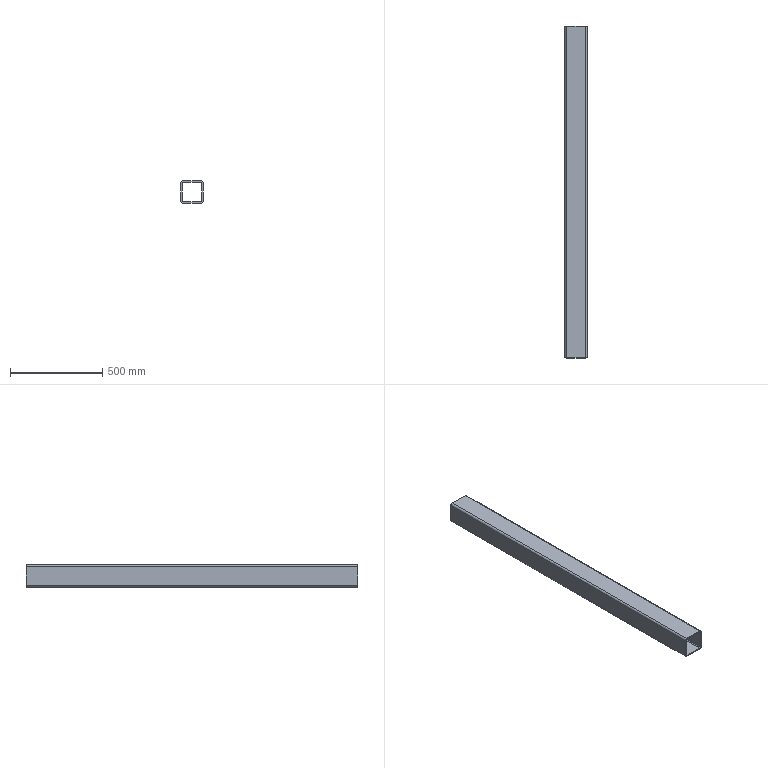Part | SolidWorks | features Extrusion 1 | 1 solid | 18 faces | box 120 x 1800 x 120 mm | volume 4795009 mm3 | plane 10 | cylinder 8 | commonest cylinder face diameters 8 x4 20 x4
STEP:
#1=CARTESIAN_POINT('',(-60.,1800.,50.));
#2=VERTEX_POINT('',#1);
#3=CARTESIAN_POINT('',(-50.,1800.,60.));
#4=VERTEX_POINT('',#3);
#5=CARTESIAN_POINT('',(-50.,1800.,50.));
#6=DIRECTION('',(0.,1.,0.));
#7=DIRECTION('',(0.,0.,-1.));
#8=AXIS2_PLACEMENT_3D('',#5,#6,#7);
#9=CIRCLE('',#8,10.);
#10=EDGE_CURVE('',#2,#4,#9,.T.);
#11=ORIENTED_EDGE('',*,*,#10,.T.);
#12=CARTESIAN_POINT('',(50.,1800.,60.));
#13=VERTEX_POINT('',#12);
#14=CARTESIAN_POINT('',(-50.,1800.,60.));
#15=DIRECTION('',(1.,0.,0.));
#16=VECTOR('',#15,1000.);
#17=LINE('',#14,#16);
#18=EDGE_CURVE('',#4,#13,#17,.T.);
#19=ORIENTED_EDGE('',*,*,#18,.T.);
#20=CARTESIAN_POINT('',(60.,1800.,50.));
#21=VERTEX_POINT('',#20);
#22=CARTESIAN_POINT('',(50.,1800.,50.));
#23=DIRECTION('',(0.,1.,0.));
#24=DIRECTION('',(0.,0.,1.));
#25=AXIS2_PLACEMENT_3D('',#22,#23,#24);
#26=CIRCLE('',#25,10.);
#27=EDGE_CURVE('',#13,#21,#26,.T.);
#28=ORIENTED_EDGE('',*,*,#27,.T.);
#29=CARTESIAN_POINT('',(60.,1800.,-50.));
#30=VERTEX_POINT('',#29);
#31=CARTESIAN_POINT('',(60.,1800.,50.));
#32=DIRECTION('',(0.,0.,-1.));
#33=VECTOR('',#32,1000.);
#34=LINE('',#31,#33);
#35=EDGE_CURVE('',#21,#30,#34,.T.);
#36=ORIENTED_EDGE('',*,*,#35,.T.);
#37=CARTESIAN_POINT('',(50.,1800.,-60.));
#38=VERTEX_POINT('',#37);
#39=CARTESIAN_POINT('',(50.,1800.,-50.));
#40=DIRECTION('',(0.,1.,0.));
#41=DIRECTION('',(0.,0.,-1.));
#42=AXIS2_PLACEMENT_3D('',#39,#40,#41);
#43=CIRCLE('',#42,10.);
#44=EDGE_CURVE('',#30,#38,#43,.T.);
#45=ORIENTED_EDGE('',*,*,#44,.T.);
#46=CARTESIAN_POINT('',(-50.,1800.,-60.));
#47=VERTEX_POINT('',#46);
#48=CARTESIAN_POINT('',(-50.,1800.,-60.));
#49=DIRECTION('',(-1.,0.,0.));
#50=VECTOR('',#49,1000.);
#51=LINE('',#48,#50);
#52=EDGE_CURVE('',#38,#47,#51,.T.);
#53=ORIENTED_EDGE('',*,*,#52,.T.);
#54=CARTESIAN_POINT('',(-60.,1800.,-50.));
#55=VERTEX_POINT('',#54);
#56=CARTESIAN_POINT('',(-50.,1800.,-50.));
#57=DIRECTION('',(0.,1.,0.));
#58=DIRECTION('',(0.,0.,-1.));
#59=AXIS2_PLACEMENT_3D('',#56,#57,#58);
#60=CIRCLE('',#59,10.);
#61=EDGE_CURVE('',#47,#55,#60,.T.);
#62=ORIENTED_EDGE('',*,*,#61,.T.);
#63=CARTESIAN_POINT('',(-60.,1800.,50.));
#64=DIRECTION('',(0.,0.,1.));
#65=VECTOR('',#64,1000.);
#66=LINE('',#63,#65);
#67=EDGE_CURVE('',#55,#2,#66,.T.);
#68=ORIENTED_EDGE('',*,*,#67,.T.);
#69=EDGE_LOOP('',(#11,#19,#28,#36,#45,#53,#62,#68));
#70=FACE_OUTER_BOUND('',#69,.T.);
#71=CARTESIAN_POINT('',(-54.,1800.,50.));
#72=VERTEX_POINT('',#71);
#73=CARTESIAN_POINT('',(-50.,1800.,54.));
#74=VERTEX_POINT('',#73);
#75=CARTESIAN_POINT('',(-50.,1800.,50.));
#76=DIRECTION('',(0.,1.,0.));
#77=DIRECTION('',(0.,0.,-1.));
#78=AXIS2_PLACEMENT_3D('',#75,#76,#77);
#79=CIRCLE('',#78,4.);
#80=EDGE_CURVE('',#72,#74,#79,.T.);
#81=ORIENTED_EDGE('',*,*,#80,.F.);
#82=CARTESIAN_POINT('',(-54.,1800.,-50.));
#83=VERTEX_POINT('',#82);
#84=CARTESIAN_POINT('',(-54.,1800.,50.));
#85=DIRECTION('',(0.,0.,1.));
#86=VECTOR('',#85,1000.);
#87=LINE('',#84,#86);
#88=EDGE_CURVE('',#83,#72,#87,.T.);
#89=ORIENTED_EDGE('',*,*,#88,.F.);
#90=CARTESIAN_POINT('',(-50.,1800.,-54.));
#91=VERTEX_POINT('',#90);
#92=CARTESIAN_POINT('',(-50.,1800.,-50.));
#93=DIRECTION('',(0.,1.,0.));
#94=DIRECTION('',(0.,0.,-1.));
#95=AXIS2_PLACEMENT_3D('',#92,#93,#94);
#96=CIRCLE('',#95,4.);
#97=EDGE_CURVE('',#91,#83,#96,.T.);
#98=ORIENTED_EDGE('',*,*,#97,.F.);
#99=CARTESIAN_POINT('',(50.,1800.,-54.));
#100=VERTEX_POINT('',#99);
#101=CARTESIAN_POINT('',(-50.,1800.,-54.));
#102=DIRECTION('',(-1.,0.,0.));
#103=VECTOR('',#102,1000.);
#104=LINE('',#101,#103);
#105=EDGE_CURVE('',#100,#91,#104,.T.);
#106=ORIENTED_EDGE('',*,*,#105,.F.);
#107=CARTESIAN_POINT('',(54.,1800.,-50.));
#108=VERTEX_POINT('',#107);
#109=CARTESIAN_POINT('',(50.,1800.,-50.));
#110=DIRECTION('',(0.,1.,0.));
#111=DIRECTION('',(0.,0.,-1.));
#112=AXIS2_PLACEMENT_3D('',#109,#110,#111);
#113=CIRCLE('',#112,4.);
#114=EDGE_CURVE('',#108,#100,#113,.T.);
#115=ORIENTED_EDGE('',*,*,#114,.F.);
#116=CARTESIAN_POINT('',(54.,1800.,50.));
#117=VERTEX_POINT('',#116);
#118=CARTESIAN_POINT('',(54.,1800.,50.));
#119=DIRECTION('',(0.,0.,-1.));
#120=VECTOR('',#119,1000.);
#121=LINE('',#118,#120);
#122=EDGE_CURVE('',#117,#108,#121,.T.);
#123=ORIENTED_EDGE('',*,*,#122,.F.);
#124=CARTESIAN_POINT('',(50.,1800.,54.));
#125=VERTEX_POINT('',#124);
#126=CARTESIAN_POINT('',(50.,1800.,50.));
#127=DIRECTION('',(0.,1.,0.));
#128=DIRECTION('',(0.,0.,1.));
#129=AXIS2_PLACEMENT_3D('',#126,#127,#128);
#130=CIRCLE('',#129,4.);
#131=EDGE_CURVE('',#125,#117,#130,.T.);
#132=ORIENTED_EDGE('',*,*,#131,.F.);
#133=CARTESIAN_POINT('',(-50.,1800.,54.));
#134=DIRECTION('',(1.,0.,0.));
#135=VECTOR('',#134,1000.);
#136=LINE('',#133,#135);
#137=EDGE_CURVE('',#74,#125,#136,.T.);
#138=ORIENTED_EDGE('',*,*,#137,.F.);
#139=EDGE_LOOP('',(#81,#89,#98,#106,#115,#123,#132,#138));
#140=FACE_BOUND('',#139,.T.);
#141=CARTESIAN_POINT('',(-50.,1800.,50.));
#142=DIRECTION('',(0.,-1.,0.));
#143=DIRECTION('',(0.,0.,-1.));
#144=AXIS2_PLACEMENT_3D('',#141,#142,#143);
#145=PLANE('',#144);
#146=ADVANCED_FACE('',(#70,#140),#145,.F.);
#147=CARTESIAN_POINT('',(-60.,0.,50.));
#148=VERTEX_POINT('',#147);
#149=CARTESIAN_POINT('',(-50.,0.,60.));
#150=VERTEX_POINT('',#149);
#151=CARTESIAN_POINT('',(-50.,0.,50.));
#152=DIRECTION('',(0.,1.,0.));
#153=DIRECTION('',(0.,0.,-1.));
#154=AXIS2_PLACEMENT_3D('',#151,#152,#153);
#155=CIRCLE('',#154,10.);
#156=EDGE_CURVE('',#148,#150,#155,.T.);
#157=ORIENTED_EDGE('',*,*,#156,.F.);
#158=CARTESIAN_POINT('',(-60.,0.,-50.));
#159=VERTEX_POINT('',#158);
#160=CARTESIAN_POINT('',(-60.,0.,50.));
#161=DIRECTION('',(0.,0.,1.));
#162=VECTOR('',#161,1000.);
#163=LINE('',#160,#162);
#164=EDGE_CURVE('',#159,#148,#163,.T.);
#165=ORIENTED_EDGE('',*,*,#164,.F.);
#166=CARTESIAN_POINT('',(-50.,0.,-60.));
#167=VERTEX_POINT('',#166);
#168=CARTESIAN_POINT('',(-50.,0.,-50.));
#169=DIRECTION('',(0.,1.,0.));
#170=DIRECTION('',(0.,0.,-1.));
#171=AXIS2_PLACEMENT_3D('',#168,#169,#170);
#172=CIRCLE('',#171,10.);
#173=EDGE_CURVE('',#167,#159,#172,.T.);
#174=ORIENTED_EDGE('',*,*,#173,.F.);
#175=CARTESIAN_POINT('',(50.,0.,-60.));
#176=VERTEX_POINT('',#175);
#177=CARTESIAN_POINT('',(-50.,0.,-60.));
#178=DIRECTION('',(-1.,0.,0.));
#179=VECTOR('',#178,1000.);
#180=LINE('',#177,#179);
#181=EDGE_CURVE('',#176,#167,#180,.T.);
#182=ORIENTED_EDGE('',*,*,#181,.F.);
#183=CARTESIAN_POINT('',(60.,0.,-50.));
#184=VERTEX_POINT('',#183);
#185=CARTESIAN_POINT('',(50.,0.,-50.));
#186=DIRECTION('',(0.,1.,0.));
#187=DIRECTION('',(0.,0.,-1.));
#188=AXIS2_PLACEMENT_3D('',#185,#186,#187);
#189=CIRCLE('',#188,10.);
#190=EDGE_CURVE('',#184,#176,#189,.T.);
#191=ORIENTED_EDGE('',*,*,#190,.F.);
#192=CARTESIAN_POINT('',(60.,0.,50.));
#193=VERTEX_POINT('',#192);
#194=CARTESIAN_POINT('',(60.,0.,50.));
#195=DIRECTION('',(0.,0.,-1.));
#196=VECTOR('',#195,1000.);
#197=LINE('',#194,#196);
#198=EDGE_CURVE('',#193,#184,#197,.T.);
#199=ORIENTED_EDGE('',*,*,#198,.F.);
#200=CARTESIAN_POINT('',(50.,0.,60.));
#201=VERTEX_POINT('',#200);
#202=CARTESIAN_POINT('',(50.,0.,50.));
#203=DIRECTION('',(0.,1.,0.));
#204=DIRECTION('',(0.,0.,1.));
#205=AXIS2_PLACEMENT_3D('',#202,#203,#204);
#206=CIRCLE('',#205,10.);
#207=EDGE_CURVE('',#201,#193,#206,.T.);
#208=ORIENTED_EDGE('',*,*,#207,.F.);
#209=CARTESIAN_POINT('',(-50.,0.,60.));
#210=DIRECTION('',(1.,0.,0.));
#211=VECTOR('',#210,1000.);
#212=LINE('',#209,#211);
#213=EDGE_CURVE('',#150,#201,#212,.T.);
#214=ORIENTED_EDGE('',*,*,#213,.F.);
#215=EDGE_LOOP('',(#157,#165,#174,#182,#191,#199,#208,#214));
#216=FACE_OUTER_BOUND('',#215,.T.);
#217=CARTESIAN_POINT('',(-54.,0.,-50.));
#218=VERTEX_POINT('',#217);
#219=CARTESIAN_POINT('',(-54.,0.,50.));
#220=VERTEX_POINT('',#219);
#221=CARTESIAN_POINT('',(-54.,0.,50.));
#222=DIRECTION('',(0.,0.,1.));
#223=VECTOR('',#222,1000.);
#224=LINE('',#221,#223);
#225=EDGE_CURVE('',#218,#220,#224,.T.);
#226=ORIENTED_EDGE('',*,*,#225,.T.);
#227=CARTESIAN_POINT('',(-50.,0.,54.));
#228=VERTEX_POINT('',#227);
#229=CARTESIAN_POINT('',(-50.,0.,50.));
#230=DIRECTION('',(0.,1.,0.));
#231=DIRECTION('',(0.,0.,-1.));
#232=AXIS2_PLACEMENT_3D('',#229,#230,#231);
#233=CIRCLE('',#232,4.);
#234=EDGE_CURVE('',#220,#228,#233,.T.);
#235=ORIENTED_EDGE('',*,*,#234,.T.);
#236=CARTESIAN_POINT('',(50.,0.,54.));
#237=VERTEX_POINT('',#236);
#238=CARTESIAN_POINT('',(-50.,0.,54.));
#239=DIRECTION('',(1.,0.,0.));
#240=VECTOR('',#239,1000.);
#241=LINE('',#238,#240);
#242=EDGE_CURVE('',#228,#237,#241,.T.);
#243=ORIENTED_EDGE('',*,*,#242,.T.);
#244=CARTESIAN_POINT('',(54.,0.,50.));
#245=VERTEX_POINT('',#244);
#246=CARTESIAN_POINT('',(50.,0.,50.));
#247=DIRECTION('',(0.,1.,0.));
#248=DIRECTION('',(0.,0.,1.));
#249=AXIS2_PLACEMENT_3D('',#246,#247,#248);
#250=CIRCLE('',#249,4.);
#251=EDGE_CURVE('',#237,#245,#250,.T.);
#252=ORIENTED_EDGE('',*,*,#251,.T.);
#253=CARTESIAN_POINT('',(54.,0.,-50.));
#254=VERTEX_POINT('',#253);
#255=CARTESIAN_POINT('',(54.,0.,50.));
#256=DIRECTION('',(0.,0.,-1.));
#257=VECTOR('',#256,1000.);
#258=LINE('',#255,#257);
#259=EDGE_CURVE('',#245,#254,#258,.T.);
#260=ORIENTED_EDGE('',*,*,#259,.T.);
#261=CARTESIAN_POINT('',(50.,0.,-54.));
#262=VERTEX_POINT('',#261);
#263=CARTESIAN_POINT('',(50.,0.,-50.));
#264=DIRECTION('',(0.,1.,0.));
#265=DIRECTION('',(0.,0.,-1.));
#266=AXIS2_PLACEMENT_3D('',#263,#264,#265);
#267=CIRCLE('',#266,4.);
#268=EDGE_CURVE('',#254,#262,#267,.T.);
#269=ORIENTED_EDGE('',*,*,#268,.T.);
#270=CARTESIAN_POINT('',(-50.,0.,-54.));
#271=VERTEX_POINT('',#270);
#272=CARTESIAN_POINT('',(-50.,0.,-54.));
#273=DIRECTION('',(-1.,0.,0.));
#274=VECTOR('',#273,1000.);
#275=LINE('',#272,#274);
#276=EDGE_CURVE('',#262,#271,#275,.T.);
#277=ORIENTED_EDGE('',*,*,#276,.T.);
#278=CARTESIAN_POINT('',(-50.,0.,-50.));
#279=DIRECTION('',(0.,1.,0.));
#280=DIRECTION('',(0.,0.,-1.));
#281=AXIS2_PLACEMENT_3D('',#278,#279,#280);
#282=CIRCLE('',#281,4.);
#283=EDGE_CURVE('',#271,#218,#282,.T.);
#284=ORIENTED_EDGE('',*,*,#283,.T.);
#285=EDGE_LOOP('',(#226,#235,#243,#252,#260,#269,#277,#284));
#286=FACE_BOUND('',#285,.T.);
#287=CARTESIAN_POINT('',(-50.,0.,50.));
#288=DIRECTION('',(0.,-1.,0.));
#289=DIRECTION('',(0.,0.,-1.));
#290=AXIS2_PLACEMENT_3D('',#287,#288,#289);
#291=PLANE('',#290);
#292=ADVANCED_FACE('',(#216,#286),#291,.T.);
#293=ORIENTED_EDGE('',*,*,#156,.T.);
#294=CARTESIAN_POINT('',(-50.,1800.,60.));
#295=DIRECTION('',(0.,-1.,0.));
#296=VECTOR('',#295,1000.);
#297=LINE('',#294,#296);
#298=EDGE_CURVE('',#4,#150,#297,.T.);
#299=ORIENTED_EDGE('',*,*,#298,.F.);
#300=ORIENTED_EDGE('',*,*,#10,.F.);
#301=CARTESIAN_POINT('',(-60.,1800.,50.));
#302=DIRECTION('',(0.,-1.,0.));
#303=VECTOR('',#302,1000.);
#304=LINE('',#301,#303);
#305=EDGE_CURVE('',#2,#148,#304,.T.);
#306=ORIENTED_EDGE('',*,*,#305,.T.);
#307=EDGE_LOOP('',(#293,#299,#300,#306));
#308=FACE_OUTER_BOUND('',#307,.T.);
#309=CARTESIAN_POINT('',(-50.,1800.,50.));
#310=DIRECTION('',(0.,-1.,0.));
#311=DIRECTION('',(0.,0.,-1.));
#312=AXIS2_PLACEMENT_3D('',#309,#310,#311);
#313=CYLINDRICAL_SURFACE('',#312,10.);
#314=ADVANCED_FACE('',(#308),#313,.T.);
#315=ORIENTED_EDGE('',*,*,#213,.T.);
#316=CARTESIAN_POINT('',(50.,1800.,60.));
#317=DIRECTION('',(0.,-1.,0.));
#318=VECTOR('',#317,1000.);
#319=LINE('',#316,#318);
#320=EDGE_CURVE('',#13,#201,#319,.T.);
#321=ORIENTED_EDGE('',*,*,#320,.F.);
#322=ORIENTED_EDGE('',*,*,#18,.F.);
#323=ORIENTED_EDGE('',*,*,#298,.T.);
#324=EDGE_LOOP('',(#315,#321,#322,#323));
#325=FACE_OUTER_BOUND('',#324,.T.);
#326=CARTESIAN_POINT('',(-50.,1800.,60.));
#327=DIRECTION('',(0.,0.,-1.));
#328=DIRECTION('',(-1.,0.,0.));
#329=AXIS2_PLACEMENT_3D('',#326,#327,#328);
#330=PLANE('',#329);
#331=ADVANCED_FACE('',(#325),#330,.F.);
#332=ORIENTED_EDGE('',*,*,#207,.T.);
#333=CARTESIAN_POINT('',(60.,1800.,50.));
#334=DIRECTION('',(0.,-1.,0.));
#335=VECTOR('',#334,1000.);
#336=LINE('',#333,#335);
#337=EDGE_CURVE('',#21,#193,#336,.T.);
#338=ORIENTED_EDGE('',*,*,#337,.F.);
#339=ORIENTED_EDGE('',*,*,#27,.F.);
#340=ORIENTED_EDGE('',*,*,#320,.T.);
#341=EDGE_LOOP('',(#332,#338,#339,#340));
#342=FACE_OUTER_BOUND('',#341,.T.);
#343=CARTESIAN_POINT('',(50.,1800.,50.));
#344=DIRECTION('',(0.,-1.,0.));
#345=DIRECTION('',(0.,0.,-1.));
#346=AXIS2_PLACEMENT_3D('',#343,#344,#345);
#347=CYLINDRICAL_SURFACE('',#346,10.);
#348=ADVANCED_FACE('',(#342),#347,.T.);
#349=ORIENTED_EDGE('',*,*,#198,.T.);
#350=CARTESIAN_POINT('',(60.,1800.,-50.));
#351=DIRECTION('',(0.,-1.,0.));
#352=VECTOR('',#351,1000.);
#353=LINE('',#350,#352);
#354=EDGE_CURVE('',#30,#184,#353,.T.);
#355=ORIENTED_EDGE('',*,*,#354,.F.);
#356=ORIENTED_EDGE('',*,*,#35,.F.);
#357=ORIENTED_EDGE('',*,*,#337,.T.);
#358=EDGE_LOOP('',(#349,#355,#356,#357));
#359=FACE_OUTER_BOUND('',#358,.T.);
#360=CARTESIAN_POINT('',(60.,1800.,50.));
#361=DIRECTION('',(-1.,0.,0.));
#362=DIRECTION('',(0.,0.,1.));
#363=AXIS2_PLACEMENT_3D('',#360,#361,#362);
#364=PLANE('',#363);
#365=ADVANCED_FACE('',(#359),#364,.F.);
#366=ORIENTED_EDGE('',*,*,#190,.T.);
#367=CARTESIAN_POINT('',(50.,1800.,-60.));
#368=DIRECTION('',(0.,-1.,0.));
#369=VECTOR('',#368,1000.);
#370=LINE('',#367,#369);
#371=EDGE_CURVE('',#38,#176,#370,.T.);
#372=ORIENTED_EDGE('',*,*,#371,.F.);
#373=ORIENTED_EDGE('',*,*,#44,.F.);
#374=ORIENTED_EDGE('',*,*,#354,.T.);
#375=EDGE_LOOP('',(#366,#372,#373,#374));
#376=FACE_OUTER_BOUND('',#375,.T.);
#377=CARTESIAN_POINT('',(50.,1800.,-50.));
#378=DIRECTION('',(0.,-1.,0.));
#379=DIRECTION('',(0.,0.,-1.));
#380=AXIS2_PLACEMENT_3D('',#377,#378,#379);
#381=CYLINDRICAL_SURFACE('',#380,10.);
#382=ADVANCED_FACE('',(#376),#381,.T.);
#383=ORIENTED_EDGE('',*,*,#181,.T.);
#384=CARTESIAN_POINT('',(-50.,1800.,-60.));
#385=DIRECTION('',(0.,-1.,0.));
#386=VECTOR('',#385,1000.);
#387=LINE('',#384,#386);
#388=EDGE_CURVE('',#47,#167,#387,.T.);
#389=ORIENTED_EDGE('',*,*,#388,.F.);
#390=ORIENTED_EDGE('',*,*,#52,.F.);
#391=ORIENTED_EDGE('',*,*,#371,.T.);
#392=EDGE_LOOP('',(#383,#389,#390,#391));
#393=FACE_OUTER_BOUND('',#392,.T.);
#394=CARTESIAN_POINT('',(-50.,1800.,-60.));
#395=DIRECTION('',(0.,0.,1.));
#396=DIRECTION('',(1.,0.,0.));
#397=AXIS2_PLACEMENT_3D('',#394,#395,#396);
#398=PLANE('',#397);
#399=ADVANCED_FACE('',(#393),#398,.F.);
#400=ORIENTED_EDGE('',*,*,#173,.T.);
#401=CARTESIAN_POINT('',(-60.,1800.,-50.));
#402=DIRECTION('',(0.,-1.,0.));
#403=VECTOR('',#402,1000.);
#404=LINE('',#401,#403);
#405=EDGE_CURVE('',#55,#159,#404,.T.);
#406=ORIENTED_EDGE('',*,*,#405,.F.);
#407=ORIENTED_EDGE('',*,*,#61,.F.);
#408=ORIENTED_EDGE('',*,*,#388,.T.);
#409=EDGE_LOOP('',(#400,#406,#407,#408));
#410=FACE_OUTER_BOUND('',#409,.T.);
#411=CARTESIAN_POINT('',(-50.,1800.,-50.));
#412=DIRECTION('',(0.,-1.,0.));
#413=DIRECTION('',(0.,0.,-1.));
#414=AXIS2_PLACEMENT_3D('',#411,#412,#413);
#415=CYLINDRICAL_SURFACE('',#414,10.);
#416=ADVANCED_FACE('',(#410),#415,.T.);
#417=ORIENTED_EDGE('',*,*,#164,.T.);
#418=ORIENTED_EDGE('',*,*,#305,.F.);
#419=ORIENTED_EDGE('',*,*,#67,.F.);
#420=ORIENTED_EDGE('',*,*,#405,.T.);
#421=EDGE_LOOP('',(#417,#418,#419,#420));
#422=FACE_OUTER_BOUND('',#421,.T.);
#423=CARTESIAN_POINT('',(-60.,1800.,50.));
#424=DIRECTION('',(1.,0.,0.));
#425=DIRECTION('',(0.,0.,-1.));
#426=AXIS2_PLACEMENT_3D('',#423,#424,#425);
#427=PLANE('',#426);
#428=ADVANCED_FACE('',(#422),#427,.F.);
#429=ORIENTED_EDGE('',*,*,#234,.F.);
#430=CARTESIAN_POINT('',(-54.,1800.,50.));
#431=DIRECTION('',(0.,-1.,0.));
#432=VECTOR('',#431,1000.);
#433=LINE('',#430,#432);
#434=EDGE_CURVE('',#72,#220,#433,.T.);
#435=ORIENTED_EDGE('',*,*,#434,.F.);
#436=ORIENTED_EDGE('',*,*,#80,.T.);
#437=CARTESIAN_POINT('',(-50.,1800.,54.));
#438=DIRECTION('',(0.,-1.,0.));
#439=VECTOR('',#438,1000.);
#440=LINE('',#437,#439);
#441=EDGE_CURVE('',#74,#228,#440,.T.);
#442=ORIENTED_EDGE('',*,*,#441,.T.);
#443=EDGE_LOOP('',(#429,#435,#436,#442));
#444=FACE_OUTER_BOUND('',#443,.T.);
#445=CARTESIAN_POINT('',(-50.,1800.,50.));
#446=DIRECTION('',(0.,-1.,0.));
#447=DIRECTION('',(0.,0.,-1.));
#448=AXIS2_PLACEMENT_3D('',#445,#446,#447);
#449=CYLINDRICAL_SURFACE('',#448,4.);
#450=ADVANCED_FACE('',(#444),#449,.F.);
#451=ORIENTED_EDGE('',*,*,#242,.F.);
#452=ORIENTED_EDGE('',*,*,#441,.F.);
#453=ORIENTED_EDGE('',*,*,#137,.T.);
#454=CARTESIAN_POINT('',(50.,1800.,54.));
#455=DIRECTION('',(0.,-1.,0.));
#456=VECTOR('',#455,1000.);
#457=LINE('',#454,#456);
#458=EDGE_CURVE('',#125,#237,#457,.T.);
#459=ORIENTED_EDGE('',*,*,#458,.T.);
#460=EDGE_LOOP('',(#451,#452,#453,#459));
#461=FACE_OUTER_BOUND('',#460,.T.);
#462=CARTESIAN_POINT('',(-50.,1800.,54.));
#463=DIRECTION('',(0.,0.,-1.));
#464=DIRECTION('',(-1.,0.,0.));
#465=AXIS2_PLACEMENT_3D('',#462,#463,#464);
#466=PLANE('',#465);
#467=ADVANCED_FACE('',(#461),#466,.T.);
#468=ORIENTED_EDGE('',*,*,#251,.F.);
#469=ORIENTED_EDGE('',*,*,#458,.F.);
#470=ORIENTED_EDGE('',*,*,#131,.T.);
#471=CARTESIAN_POINT('',(54.,1800.,50.));
#472=DIRECTION('',(0.,-1.,0.));
#473=VECTOR('',#472,1000.);
#474=LINE('',#471,#473);
#475=EDGE_CURVE('',#117,#245,#474,.T.);
#476=ORIENTED_EDGE('',*,*,#475,.T.);
#477=EDGE_LOOP('',(#468,#469,#470,#476));
#478=FACE_OUTER_BOUND('',#477,.T.);
#479=CARTESIAN_POINT('',(50.,1800.,50.));
#480=DIRECTION('',(0.,-1.,0.));
#481=DIRECTION('',(0.,0.,-1.));
#482=AXIS2_PLACEMENT_3D('',#479,#480,#481);
#483=CYLINDRICAL_SURFACE('',#482,4.);
#484=ADVANCED_FACE('',(#478),#483,.F.);
#485=ORIENTED_EDGE('',*,*,#259,.F.);
#486=ORIENTED_EDGE('',*,*,#475,.F.);
#487=ORIENTED_EDGE('',*,*,#122,.T.);
#488=CARTESIAN_POINT('',(54.,1800.,-50.));
#489=DIRECTION('',(0.,-1.,0.));
#490=VECTOR('',#489,1000.);
#491=LINE('',#488,#490);
#492=EDGE_CURVE('',#108,#254,#491,.T.);
#493=ORIENTED_EDGE('',*,*,#492,.T.);
#494=EDGE_LOOP('',(#485,#486,#487,#493));
#495=FACE_OUTER_BOUND('',#494,.T.);
#496=CARTESIAN_POINT('',(54.,1800.,50.));
#497=DIRECTION('',(-1.,0.,0.));
#498=DIRECTION('',(0.,0.,1.));
#499=AXIS2_PLACEMENT_3D('',#496,#497,#498);
#500=PLANE('',#499);
#501=ADVANCED_FACE('',(#495),#500,.T.);
#502=ORIENTED_EDGE('',*,*,#268,.F.);
#503=ORIENTED_EDGE('',*,*,#492,.F.);
#504=ORIENTED_EDGE('',*,*,#114,.T.);
#505=CARTESIAN_POINT('',(50.,1800.,-54.));
#506=DIRECTION('',(0.,-1.,0.));
#507=VECTOR('',#506,1000.);
#508=LINE('',#505,#507);
#509=EDGE_CURVE('',#100,#262,#508,.T.);
#510=ORIENTED_EDGE('',*,*,#509,.T.);
#511=EDGE_LOOP('',(#502,#503,#504,#510));
#512=FACE_OUTER_BOUND('',#511,.T.);
#513=CARTESIAN_POINT('',(50.,1800.,-50.));
#514=DIRECTION('',(0.,-1.,0.));
#515=DIRECTION('',(0.,0.,-1.));
#516=AXIS2_PLACEMENT_3D('',#513,#514,#515);
#517=CYLINDRICAL_SURFACE('',#516,4.);
#518=ADVANCED_FACE('',(#512),#517,.F.);
#519=ORIENTED_EDGE('',*,*,#276,.F.);
#520=ORIENTED_EDGE('',*,*,#509,.F.);
#521=ORIENTED_EDGE('',*,*,#105,.T.);
#522=CARTESIAN_POINT('',(-50.,1800.,-54.));
#523=DIRECTION('',(0.,-1.,0.));
#524=VECTOR('',#523,1000.);
#525=LINE('',#522,#524);
#526=EDGE_CURVE('',#91,#271,#525,.T.);
#527=ORIENTED_EDGE('',*,*,#526,.T.);
#528=EDGE_LOOP('',(#519,#520,#521,#527));
#529=FACE_OUTER_BOUND('',#528,.T.);
#530=CARTESIAN_POINT('',(-50.,1800.,-54.));
#531=DIRECTION('',(0.,0.,1.));
#532=DIRECTION('',(1.,0.,0.));
#533=AXIS2_PLACEMENT_3D('',#530,#531,#532);
#534=PLANE('',#533);
#535=ADVANCED_FACE('',(#529),#534,.T.);
#536=ORIENTED_EDGE('',*,*,#283,.F.);
#537=ORIENTED_EDGE('',*,*,#526,.F.);
#538=ORIENTED_EDGE('',*,*,#97,.T.);
#539=CARTESIAN_POINT('',(-54.,1800.,-50.));
#540=DIRECTION('',(0.,-1.,0.));
#541=VECTOR('',#540,1000.);
#542=LINE('',#539,#541);
#543=EDGE_CURVE('',#83,#218,#542,.T.);
#544=ORIENTED_EDGE('',*,*,#543,.T.);
#545=EDGE_LOOP('',(#536,#537,#538,#544));
#546=FACE_OUTER_BOUND('',#545,.T.);
#547=CARTESIAN_POINT('',(-50.,1800.,-50.));
#548=DIRECTION('',(0.,-1.,0.));
#549=DIRECTION('',(0.,0.,-1.));
#550=AXIS2_PLACEMENT_3D('',#547,#548,#549);
#551=CYLINDRICAL_SURFACE('',#550,4.);
#552=ADVANCED_FACE('',(#546),#551,.F.);
#553=ORIENTED_EDGE('',*,*,#225,.F.);
#554=ORIENTED_EDGE('',*,*,#543,.F.);
#555=ORIENTED_EDGE('',*,*,#88,.T.);
#556=ORIENTED_EDGE('',*,*,#434,.T.);
#557=EDGE_LOOP('',(#553,#554,#555,#556));
#558=FACE_OUTER_BOUND('',#557,.T.);
#559=CARTESIAN_POINT('',(-54.,1800.,50.));
#560=DIRECTION('',(1.,0.,0.));
#561=DIRECTION('',(0.,0.,-1.));
#562=AXIS2_PLACEMENT_3D('',#559,#560,#561);
#563=PLANE('',#562);
#564=ADVANCED_FACE('',(#558),#563,.T.);
#565=CLOSED_SHELL('',(#146,#292,#314,#331,#348,#365,#382,#399,#416,#428,#450,#467,#484,#501,#518,#535,#552,#564));
#566=MANIFOLD_SOLID_BREP('',#565);
#567=CARTESIAN_POINT('',(0.,0.,0.));
#568=DIRECTION('',(0.,0.,1.));
#569=DIRECTION('',(1.,0.,0.));
#570=AXIS2_PLACEMENT_3D('',#567,#568,#569);
#571=(LENGTH_UNIT()NAMED_UNIT(*)SI_UNIT(.MILLI.,.METRE.));
#572=UNCERTAINTY_MEASURE_WITH_UNIT(LENGTH_MEASURE(0.00001),#571,'','');
#573=(NAMED_UNIT(*)PLANE_ANGLE_UNIT()SI_UNIT($,.RADIAN.));
#574=(NAMED_UNIT(*)SI_UNIT($,.STERADIAN.)SOLID_ANGLE_UNIT());
#575=(GEOMETRIC_REPRESENTATION_CONTEXT(3)GLOBAL_UNCERTAINTY_ASSIGNED_CONTEXT((#572))GLOBAL_UNIT_ASSIGNED_CONTEXT((#571,#573,#574))REPRESENTATION_CONTEXT('',''));
#576=ADVANCED_BREP_SHAPE_REPRESENTATION('',(#566,#570),#575);